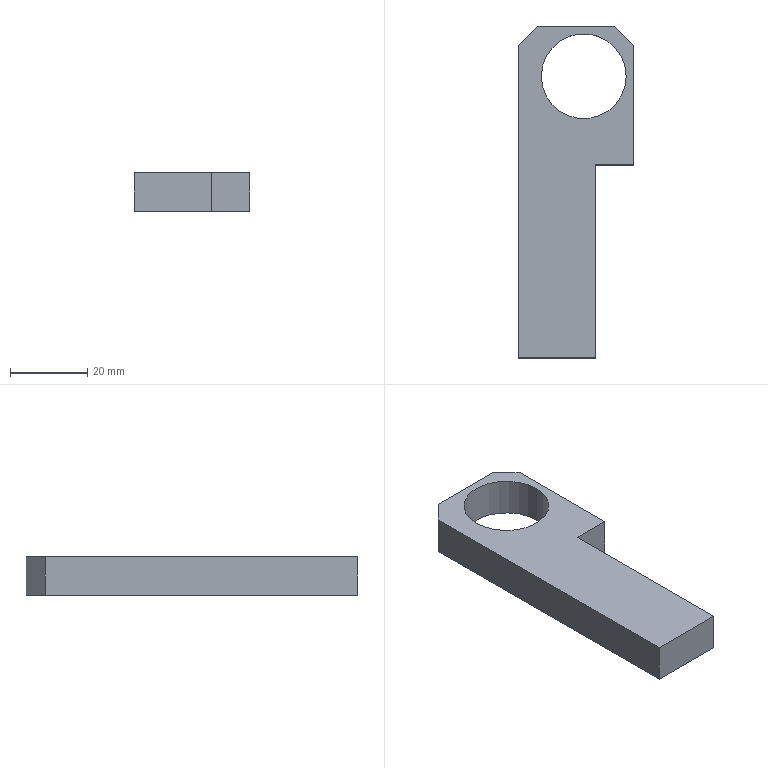Part | STEP file | A08 | 1 solid | 20 faces | box 30 x 86 x 10 mm | volume 16393 mm3 | plane 10 | cylinder 6 | cone 4 | commonest cylinder face diameters 4.2 x4 22 x2
STEP:
#1=CARTESIAN_POINT('',(0.,0.,0.));
#2=DIRECTION('',(0.,0.,1.));
#3=DIRECTION('',(1.,0.,0.));
#4=AXIS2_PLACEMENT_3D('',#1,#2,#3);
#5=CARTESIAN_POINT('',(-7.4,-13.,2.9));
#6=VERTEX_POINT('',#5);
#7=CARTESIAN_POINT('',(5.,-13.,2.9));
#8=VERTEX_POINT('',#7);
#9=CARTESIAN_POINT('',(5.,-13.,2.9));
#10=DIRECTION('',(1.,0.,0.));
#11=VECTOR('',#10,1.);
#12=LINE('',#9,#11);
#13=CARTESIAN_POINT('',(5.,-13.,5.));
#14=DIRECTION('',(1.,0.,0.));
#15=DIRECTION('',(0.,0.,-1.));
#16=AXIS2_PLACEMENT_3D('',#13,#14,#15);
#17=CYLINDRICAL_SURFACE('',#16,2.1);
#18=CARTESIAN_POINT('',(6.283,0.));
#19=DIRECTION('',(0.,1.));
#20=VECTOR('',#19,1.);
#21=LINE('',#18,#20);
#22=(GEOMETRIC_REPRESENTATION_CONTEXT(2)PARAMETRIC_REPRESENTATION_CONTEXT()REPRESENTATION_CONTEXT('',''));
#23=DEFINITIONAL_REPRESENTATION('',(#21),#22);
#24=PCURVE('',#17,#23);
#25=CARTESIAN_POINT('',(5.,-13.,5.));
#26=DIRECTION('',(1.,0.,0.));
#27=DIRECTION('',(0.,0.,-1.));
#28=AXIS2_PLACEMENT_3D('',#25,#26,#27);
#29=CYLINDRICAL_SURFACE('',#28,2.1);
#30=CARTESIAN_POINT('',(0.,0.));
#31=DIRECTION('',(0.,1.));
#32=VECTOR('',#31,1.);
#33=LINE('',#30,#32);
#34=(GEOMETRIC_REPRESENTATION_CONTEXT(2)PARAMETRIC_REPRESENTATION_CONTEXT()REPRESENTATION_CONTEXT('',''));
#35=DEFINITIONAL_REPRESENTATION('',(#33),#34);
#36=PCURVE('',#29,#35);
#37=SURFACE_CURVE('',#12,(#24,#36),.PCURVE_S1.);
#38=EDGE_CURVE('',#6,#8,#37,.T.);
#39=ORIENTED_EDGE('',*,*,#38,.T.);
#40=CARTESIAN_POINT('',(5.,-13.,7.1));
#41=VERTEX_POINT('',#40);
#42=CARTESIAN_POINT('',(5.,-13.,5.));
#43=DIRECTION('',(1.,0.,0.));
#44=DIRECTION('',(0.,0.,-1.));
#45=AXIS2_PLACEMENT_3D('',#42,#43,#44);
#46=CIRCLE('',#45,2.1);
#47=CARTESIAN_POINT('',(0.,0.));
#48=DIRECTION('',(1.,0.));
#49=VECTOR('',#48,1.);
#50=LINE('',#47,#49);
#51=(GEOMETRIC_REPRESENTATION_CONTEXT(2)PARAMETRIC_REPRESENTATION_CONTEXT()REPRESENTATION_CONTEXT('',''));
#52=DEFINITIONAL_REPRESENTATION('',(#50),#51);
#53=PCURVE('',#17,#52);
#54=CARTESIAN_POINT('',(5.,-43.,0.));
#55=DIRECTION('',(-1.,0.,0.));
#56=DIRECTION('',(0.,0.,1.));
#57=AXIS2_PLACEMENT_3D('',#54,#55,#56);
#58=PLANE('',#57);
#59=CARTESIAN_POINT('',(2.9,30.));
#60=CARTESIAN_POINT('',(2.9,33.637));
#61=CARTESIAN_POINT('',(6.05,31.819));
#62=CARTESIAN_POINT('',(9.2,30.));
#63=CARTESIAN_POINT('',(6.05,28.181));
#64=CARTESIAN_POINT('',(2.9,26.363));
#65=CARTESIAN_POINT('',(2.9,30.));
#66=(BOUNDED_CURVE()B_SPLINE_CURVE(2,(#59,#60,#61,#62,#63,#64,#65),.UNSPECIFIED.,.T.,.F.)B_SPLINE_CURVE_WITH_KNOTS((1,2,2,2,2,1),(-2.094,0.,2.094,4.189,6.283,8.378),.UNSPECIFIED.)CURVE()GEOMETRIC_REPRESENTATION_ITEM()RATIONAL_B_SPLINE_CURVE((1.,0.5,1.,0.5,1.,0.5,1.))REPRESENTATION_ITEM(''));
#67=(GEOMETRIC_REPRESENTATION_CONTEXT(2)PARAMETRIC_REPRESENTATION_CONTEXT()REPRESENTATION_CONTEXT('',''));
#68=DEFINITIONAL_REPRESENTATION('',(#66),#67);
#69=PCURVE('',#58,#68);
#70=SURFACE_CURVE('',#46,(#53,#69),.PCURVE_S1.);
#71=EDGE_CURVE('',#41,#8,#70,.T.);
#72=ORIENTED_EDGE('',*,*,#71,.F.);
#73=CARTESIAN_POINT('',(-7.4,-13.,7.1));
#74=VERTEX_POINT('',#73);
#75=CARTESIAN_POINT('',(5.,-13.,7.1));
#76=DIRECTION('',(1.,0.,0.));
#77=VECTOR('',#76,1.);
#78=LINE('',#75,#77);
#79=CARTESIAN_POINT('',(3.142,0.));
#80=DIRECTION('',(0.,1.));
#81=VECTOR('',#80,1.);
#82=LINE('',#79,#81);
#83=(GEOMETRIC_REPRESENTATION_CONTEXT(2)PARAMETRIC_REPRESENTATION_CONTEXT()REPRESENTATION_CONTEXT('',''));
#84=DEFINITIONAL_REPRESENTATION('',(#82),#83);
#85=PCURVE('',#17,#84);
#86=CARTESIAN_POINT('',(3.142,0.));
#87=DIRECTION('',(0.,1.));
#88=VECTOR('',#87,1.);
#89=LINE('',#86,#88);
#90=(GEOMETRIC_REPRESENTATION_CONTEXT(2)PARAMETRIC_REPRESENTATION_CONTEXT()REPRESENTATION_CONTEXT('',''));
#91=DEFINITIONAL_REPRESENTATION('',(#89),#90);
#92=PCURVE('',#29,#91);
#93=SURFACE_CURVE('',#78,(#85,#92),.PCURVE_S1.);
#94=EDGE_CURVE('',#74,#41,#93,.T.);
#95=ORIENTED_EDGE('',*,*,#94,.F.);
#96=CARTESIAN_POINT('',(-7.4,-13.,5.));
#97=DIRECTION('',(1.,0.,0.));
#98=DIRECTION('',(0.,0.,-1.));
#99=AXIS2_PLACEMENT_3D('',#96,#97,#98);
#100=CIRCLE('',#99,2.1);
#101=CARTESIAN_POINT('',(0.,-12.4));
#102=DIRECTION('',(1.,0.));
#103=VECTOR('',#102,1.);
#104=LINE('',#101,#103);
#105=(GEOMETRIC_REPRESENTATION_CONTEXT(2)PARAMETRIC_REPRESENTATION_CONTEXT()REPRESENTATION_CONTEXT('',''));
#106=DEFINITIONAL_REPRESENTATION('',(#104),#105);
#107=PCURVE('',#17,#106);
#108=CARTESIAN_POINT('',(-7.4,-13.,5.));
#109=DIRECTION('',(1.,0.,0.));
#110=DIRECTION('',(0.,0.,-1.));
#111=AXIS2_PLACEMENT_3D('',#108,#109,#110);
#112=CONICAL_SURFACE('',#111,2.1,1.03);
#113=CARTESIAN_POINT('',(0.,0.));
#114=DIRECTION('',(1.,0.));
#115=VECTOR('',#114,1.);
#116=LINE('',#113,#115);
#117=(GEOMETRIC_REPRESENTATION_CONTEXT(2)PARAMETRIC_REPRESENTATION_CONTEXT()REPRESENTATION_CONTEXT('',''));
#118=DEFINITIONAL_REPRESENTATION('',(#116),#117);
#119=PCURVE('',#112,#118);
#120=SURFACE_CURVE('',#100,(#107,#119),.PCURVE_S1.);
#121=EDGE_CURVE('',#74,#6,#120,.T.);
#122=ORIENTED_EDGE('',*,*,#121,.T.);
#123=EDGE_LOOP('',(#39,#72,#95,#122));
#124=FACE_BOUND('',#123,.F.);
#125=ADVANCED_FACE('',(#124),#17,.F.);
#126=ORIENTED_EDGE('',*,*,#121,.F.);
#127=CARTESIAN_POINT('',(-8.662,-13.,5.));
#128=VERTEX_POINT('',#127);
#129=CARTESIAN_POINT('',(-7.4,-13.,7.1));
#130=DIRECTION('',(0.515,0.,0.8572));
#131=VECTOR('',#130,1.);
#132=LINE('',#129,#131);
#133=CARTESIAN_POINT('',(3.142,0.));
#134=DIRECTION('',(0.,1.));
#135=VECTOR('',#134,1.);
#136=LINE('',#133,#135);
#137=(GEOMETRIC_REPRESENTATION_CONTEXT(2)PARAMETRIC_REPRESENTATION_CONTEXT()REPRESENTATION_CONTEXT('',''));
#138=DEFINITIONAL_REPRESENTATION('',(#136),#137);
#139=PCURVE('',#112,#138);
#140=CARTESIAN_POINT('',(-7.4,-13.,5.));
#141=DIRECTION('',(1.,0.,0.));
#142=DIRECTION('',(0.,0.,-1.));
#143=AXIS2_PLACEMENT_3D('',#140,#141,#142);
#144=CONICAL_SURFACE('',#143,2.1,1.03);
#145=CARTESIAN_POINT('',(3.142,0.));
#146=DIRECTION('',(0.,1.));
#147=VECTOR('',#146,1.);
#148=LINE('',#145,#147);
#149=(GEOMETRIC_REPRESENTATION_CONTEXT(2)PARAMETRIC_REPRESENTATION_CONTEXT()REPRESENTATION_CONTEXT('',''));
#150=DEFINITIONAL_REPRESENTATION('',(#148),#149);
#151=PCURVE('',#144,#150);
#152=SURFACE_CURVE('',#132,(#139,#151),.PCURVE_S1.);
#153=EDGE_CURVE('',#128,#74,#152,.T.);
#154=ORIENTED_EDGE('',*,*,#153,.F.);
#155=CARTESIAN_POINT('',(-7.4,-13.,2.9));
#156=DIRECTION('',(0.515,0.,-0.8572));
#157=VECTOR('',#156,1.);
#158=LINE('',#155,#157);
#159=CARTESIAN_POINT('',(6.283,0.));
#160=DIRECTION('',(0.,1.));
#161=VECTOR('',#160,1.);
#162=LINE('',#159,#161);
#163=(GEOMETRIC_REPRESENTATION_CONTEXT(2)PARAMETRIC_REPRESENTATION_CONTEXT()REPRESENTATION_CONTEXT('',''));
#164=DEFINITIONAL_REPRESENTATION('',(#162),#163);
#165=PCURVE('',#112,#164);
#166=CARTESIAN_POINT('',(0.,0.));
#167=DIRECTION('',(0.,1.));
#168=VECTOR('',#167,1.);
#169=LINE('',#166,#168);
#170=(GEOMETRIC_REPRESENTATION_CONTEXT(2)PARAMETRIC_REPRESENTATION_CONTEXT()REPRESENTATION_CONTEXT('',''));
#171=DEFINITIONAL_REPRESENTATION('',(#169),#170);
#172=PCURVE('',#144,#171);
#173=SURFACE_CURVE('',#158,(#165,#172),.PCURVE_S1.);
#174=EDGE_CURVE('',#128,#6,#173,.T.);
#175=ORIENTED_EDGE('',*,*,#174,.T.);
#176=EDGE_LOOP('',(#126,#154,#175));
#177=FACE_BOUND('',#176,.F.);
#178=ADVANCED_FACE('',(#177),#112,.F.);
#179=CARTESIAN_POINT('',(-7.4,-38.,2.9));
#180=VERTEX_POINT('',#179);
#181=CARTESIAN_POINT('',(5.,-38.,2.9));
#182=VERTEX_POINT('',#181);
#183=CARTESIAN_POINT('',(5.,-38.,2.9));
#184=DIRECTION('',(1.,0.,0.));
#185=VECTOR('',#184,1.);
#186=LINE('',#183,#185);
#187=CARTESIAN_POINT('',(5.,-38.,5.));
#188=DIRECTION('',(1.,0.,0.));
#189=DIRECTION('',(0.,0.,-1.));
#190=AXIS2_PLACEMENT_3D('',#187,#188,#189);
#191=CYLINDRICAL_SURFACE('',#190,2.1);
#192=CARTESIAN_POINT('',(6.283,0.));
#193=DIRECTION('',(0.,1.));
#194=VECTOR('',#193,1.);
#195=LINE('',#192,#194);
#196=(GEOMETRIC_REPRESENTATION_CONTEXT(2)PARAMETRIC_REPRESENTATION_CONTEXT()REPRESENTATION_CONTEXT('',''));
#197=DEFINITIONAL_REPRESENTATION('',(#195),#196);
#198=PCURVE('',#191,#197);
#199=CARTESIAN_POINT('',(5.,-38.,5.));
#200=DIRECTION('',(1.,0.,0.));
#201=DIRECTION('',(0.,0.,-1.));
#202=AXIS2_PLACEMENT_3D('',#199,#200,#201);
#203=CYLINDRICAL_SURFACE('',#202,2.1);
#204=CARTESIAN_POINT('',(0.,0.));
#205=DIRECTION('',(0.,1.));
#206=VECTOR('',#205,1.);
#207=LINE('',#204,#206);
#208=(GEOMETRIC_REPRESENTATION_CONTEXT(2)PARAMETRIC_REPRESENTATION_CONTEXT()REPRESENTATION_CONTEXT('',''));
#209=DEFINITIONAL_REPRESENTATION('',(#207),#208);
#210=PCURVE('',#203,#209);
#211=SURFACE_CURVE('',#186,(#198,#210),.PCURVE_S1.);
#212=EDGE_CURVE('',#180,#182,#211,.T.);
#213=ORIENTED_EDGE('',*,*,#212,.T.);
#214=CARTESIAN_POINT('',(5.,-38.,7.1));
#215=VERTEX_POINT('',#214);
#216=CARTESIAN_POINT('',(5.,-38.,5.));
#217=DIRECTION('',(1.,0.,0.));
#218=DIRECTION('',(0.,0.,-1.));
#219=AXIS2_PLACEMENT_3D('',#216,#217,#218);
#220=CIRCLE('',#219,2.1);
#221=CARTESIAN_POINT('',(0.,0.));
#222=DIRECTION('',(1.,0.));
#223=VECTOR('',#222,1.);
#224=LINE('',#221,#223);
#225=(GEOMETRIC_REPRESENTATION_CONTEXT(2)PARAMETRIC_REPRESENTATION_CONTEXT()REPRESENTATION_CONTEXT('',''));
#226=DEFINITIONAL_REPRESENTATION('',(#224),#225);
#227=PCURVE('',#191,#226);
#228=CARTESIAN_POINT('',(2.9,5.));
#229=CARTESIAN_POINT('',(2.9,8.637));
#230=CARTESIAN_POINT('',(6.05,6.819));
#231=CARTESIAN_POINT('',(9.2,5.));
#232=CARTESIAN_POINT('',(6.05,3.181));
#233=CARTESIAN_POINT('',(2.9,1.363));
#234=CARTESIAN_POINT('',(2.9,5.));
#235=(BOUNDED_CURVE()B_SPLINE_CURVE(2,(#228,#229,#230,#231,#232,#233,#234),.UNSPECIFIED.,.T.,.F.)B_SPLINE_CURVE_WITH_KNOTS((1,2,2,2,2,1),(-2.094,0.,2.094,4.189,6.283,8.378),.UNSPECIFIED.)CURVE()GEOMETRIC_REPRESENTATION_ITEM()RATIONAL_B_SPLINE_CURVE((1.,0.5,1.,0.5,1.,0.5,1.))REPRESENTATION_ITEM(''));
#236=(GEOMETRIC_REPRESENTATION_CONTEXT(2)PARAMETRIC_REPRESENTATION_CONTEXT()REPRESENTATION_CONTEXT('',''));
#237=DEFINITIONAL_REPRESENTATION('',(#235),#236);
#238=PCURVE('',#58,#237);
#239=SURFACE_CURVE('',#220,(#227,#238),.PCURVE_S1.);
#240=EDGE_CURVE('',#215,#182,#239,.T.);
#241=ORIENTED_EDGE('',*,*,#240,.F.);
#242=CARTESIAN_POINT('',(-7.4,-38.,7.1));
#243=VERTEX_POINT('',#242);
#244=CARTESIAN_POINT('',(5.,-38.,7.1));
#245=DIRECTION('',(1.,0.,0.));
#246=VECTOR('',#245,1.);
#247=LINE('',#244,#246);
#248=CARTESIAN_POINT('',(3.142,0.));
#249=DIRECTION('',(0.,1.));
#250=VECTOR('',#249,1.);
#251=LINE('',#248,#250);
#252=(GEOMETRIC_REPRESENTATION_CONTEXT(2)PARAMETRIC_REPRESENTATION_CONTEXT()REPRESENTATION_CONTEXT('',''));
#253=DEFINITIONAL_REPRESENTATION('',(#251),#252);
#254=PCURVE('',#191,#253);
#255=CARTESIAN_POINT('',(3.142,0.));
#256=DIRECTION('',(0.,1.));
#257=VECTOR('',#256,1.);
#258=LINE('',#255,#257);
#259=(GEOMETRIC_REPRESENTATION_CONTEXT(2)PARAMETRIC_REPRESENTATION_CONTEXT()REPRESENTATION_CONTEXT('',''));
#260=DEFINITIONAL_REPRESENTATION('',(#258),#259);
#261=PCURVE('',#203,#260);
#262=SURFACE_CURVE('',#247,(#254,#261),.PCURVE_S1.);
#263=EDGE_CURVE('',#243,#215,#262,.T.);
#264=ORIENTED_EDGE('',*,*,#263,.F.);
#265=CARTESIAN_POINT('',(-7.4,-38.,5.));
#266=DIRECTION('',(1.,0.,0.));
#267=DIRECTION('',(0.,0.,-1.));
#268=AXIS2_PLACEMENT_3D('',#265,#266,#267);
#269=CIRCLE('',#268,2.1);
#270=CARTESIAN_POINT('',(0.,-12.4));
#271=DIRECTION('',(1.,0.));
#272=VECTOR('',#271,1.);
#273=LINE('',#270,#272);
#274=(GEOMETRIC_REPRESENTATION_CONTEXT(2)PARAMETRIC_REPRESENTATION_CONTEXT()REPRESENTATION_CONTEXT('',''));
#275=DEFINITIONAL_REPRESENTATION('',(#273),#274);
#276=PCURVE('',#191,#275);
#277=CARTESIAN_POINT('',(-7.4,-38.,5.));
#278=DIRECTION('',(1.,0.,0.));
#279=DIRECTION('',(0.,0.,-1.));
#280=AXIS2_PLACEMENT_3D('',#277,#278,#279);
#281=CONICAL_SURFACE('',#280,2.1,1.03);
#282=CARTESIAN_POINT('',(0.,0.));
#283=DIRECTION('',(1.,0.));
#284=VECTOR('',#283,1.);
#285=LINE('',#282,#284);
#286=(GEOMETRIC_REPRESENTATION_CONTEXT(2)PARAMETRIC_REPRESENTATION_CONTEXT()REPRESENTATION_CONTEXT('',''));
#287=DEFINITIONAL_REPRESENTATION('',(#285),#286);
#288=PCURVE('',#281,#287);
#289=SURFACE_CURVE('',#269,(#276,#288),.PCURVE_S1.);
#290=EDGE_CURVE('',#243,#180,#289,.T.);
#291=ORIENTED_EDGE('',*,*,#290,.T.);
#292=EDGE_LOOP('',(#213,#241,#264,#291));
#293=FACE_BOUND('',#292,.F.);
#294=ADVANCED_FACE('',(#293),#191,.F.);
#295=ORIENTED_EDGE('',*,*,#290,.F.);
#296=CARTESIAN_POINT('',(-8.662,-38.,5.));
#297=VERTEX_POINT('',#296);
#298=CARTESIAN_POINT('',(-7.4,-38.,7.1));
#299=DIRECTION('',(0.515,0.,0.8572));
#300=VECTOR('',#299,1.);
#301=LINE('',#298,#300);
#302=CARTESIAN_POINT('',(3.142,-1.262));
#303=CARTESIAN_POINT('',(3.142,-1.243));
#304=CARTESIAN_POINT('',(3.142,-1.204));
#305=CARTESIAN_POINT('',(3.142,-1.147));
#306=CARTESIAN_POINT('',(3.142,-1.09));
#307=CARTESIAN_POINT('',(3.142,-1.032));
#308=CARTESIAN_POINT('',(3.142,-0.975));
#309=CARTESIAN_POINT('',(3.142,-0.9177));
#310=CARTESIAN_POINT('',(3.142,-0.8603));
#311=CARTESIAN_POINT('',(3.142,-0.803));
#312=CARTESIAN_POINT('',(3.142,-0.7456));
#313=CARTESIAN_POINT('',(3.142,-0.6883));
#314=CARTESIAN_POINT('',(3.142,-0.6309));
#315=CARTESIAN_POINT('',(3.142,-0.5735));
#316=CARTESIAN_POINT('',(3.142,-0.5162));
#317=CARTESIAN_POINT('',(3.142,-0.4588));
#318=CARTESIAN_POINT('',(3.142,-0.4015));
#319=CARTESIAN_POINT('',(3.142,-0.3441));
#320=CARTESIAN_POINT('',(3.142,-0.2868));
#321=CARTESIAN_POINT('',(3.142,-0.2294));
#322=CARTESIAN_POINT('',(3.142,-0.1721));
#323=CARTESIAN_POINT('',(3.142,-0.1147));
#324=CARTESIAN_POINT('',(3.142,-0.05735));
#325=CARTESIAN_POINT('',(3.142,-0.01912));
#326=CARTESIAN_POINT('',(3.142,0.));
#327=B_SPLINE_CURVE_WITH_KNOTS('',3,(#302,#303,#304,#305,#306,#307,#308,#309,#310,#311,#312,#313,#314,#315,#316,#317,#318,#319,#320,#321,#322,#323,#324,#325,#326),.UNSPECIFIED.,.F.,.F.,(4,1,1,1,1,1,1,1,1,1,1,1,1,1,1,1,1,1,1,1,1,1,4),(-2.45,-2.339,-2.227,-2.116,-2.004,-1.893,-1.782,-1.67,-1.559,-1.448,-1.336,-1.225,-1.114,-1.002,-0.8909,-0.7795,-0.6682,-0.5568,-0.4454,-0.3341,-0.2227,-0.1114,0.),.UNSPECIFIED.);
#328=(GEOMETRIC_REPRESENTATION_CONTEXT(2)PARAMETRIC_REPRESENTATION_CONTEXT()REPRESENTATION_CONTEXT('',''));
#329=DEFINITIONAL_REPRESENTATION('',(#327),#328);
#330=PCURVE('',#281,#329);
#331=CARTESIAN_POINT('',(-7.4,-38.,5.));
#332=DIRECTION('',(1.,0.,0.));
#333=DIRECTION('',(0.,0.,-1.));
#334=AXIS2_PLACEMENT_3D('',#331,#332,#333);
#335=CONICAL_SURFACE('',#334,2.1,1.03);
#336=CARTESIAN_POINT('',(3.142,-1.262));
#337=CARTESIAN_POINT('',(3.142,-1.243));
#338=CARTESIAN_POINT('',(3.142,-1.204));
#339=CARTESIAN_POINT('',(3.142,-1.147));
#340=CARTESIAN_POINT('',(3.142,-1.09));
#341=CARTESIAN_POINT('',(3.142,-1.032));
#342=CARTESIAN_POINT('',(3.142,-0.975));
#343=CARTESIAN_POINT('',(3.142,-0.9177));
#344=CARTESIAN_POINT('',(3.142,-0.8603));
#345=CARTESIAN_POINT('',(3.142,-0.803));
#346=CARTESIAN_POINT('',(3.142,-0.7456));
#347=CARTESIAN_POINT('',(3.142,-0.6883));
#348=CARTESIAN_POINT('',(3.142,-0.6309));
#349=CARTESIAN_POINT('',(3.142,-0.5735));
#350=CARTESIAN_POINT('',(3.142,-0.5162));
#351=CARTESIAN_POINT('',(3.142,-0.4588));
#352=CARTESIAN_POINT('',(3.142,-0.4015));
#353=CARTESIAN_POINT('',(3.142,-0.3441));
#354=CARTESIAN_POINT('',(3.142,-0.2868));
#355=CARTESIAN_POINT('',(3.142,-0.2294));
#356=CARTESIAN_POINT('',(3.142,-0.1721));
#357=CARTESIAN_POINT('',(3.142,-0.1147));
#358=CARTESIAN_POINT('',(3.142,-0.05735));
#359=CARTESIAN_POINT('',(3.142,-0.01912));
#360=CARTESIAN_POINT('',(3.142,0.));
#361=B_SPLINE_CURVE_WITH_KNOTS('',3,(#336,#337,#338,#339,#340,#341,#342,#343,#344,#345,#346,#347,#348,#349,#350,#351,#352,#353,#354,#355,#356,#357,#358,#359,#360),.UNSPECIFIED.,.F.,.F.,(4,1,1,1,1,1,1,1,1,1,1,1,1,1,1,1,1,1,1,1,1,1,4),(-2.45,-2.339,-2.227,-2.116,-2.004,-1.893,-1.782,-1.67,-1.559,-1.448,-1.336,-1.225,-1.114,-1.002,-0.8909,-0.7795,-0.6682,-0.5568,-0.4454,-0.3341,-0.2227,-0.1114,0.),.UNSPECIFIED.);
#362=(GEOMETRIC_REPRESENTATION_CONTEXT(2)PARAMETRIC_REPRESENTATION_CONTEXT()REPRESENTATION_CONTEXT('',''));
#363=DEFINITIONAL_REPRESENTATION('',(#361),#362);
#364=PCURVE('',#335,#363);
#365=SURFACE_CURVE('',#301,(#330,#364),.PCURVE_S1.);
#366=EDGE_CURVE('',#297,#243,#365,.T.);
#367=ORIENTED_EDGE('',*,*,#366,.F.);
#368=CARTESIAN_POINT('',(-7.4,-38.,2.9));
#369=DIRECTION('',(0.515,0.,-0.8572));
#370=VECTOR('',#369,1.);
#371=LINE('',#368,#370);
#372=CARTESIAN_POINT('',(6.283,0.));
#373=DIRECTION('',(0.,1.));
#374=VECTOR('',#373,1.);
#375=LINE('',#372,#374);
#376=(GEOMETRIC_REPRESENTATION_CONTEXT(2)PARAMETRIC_REPRESENTATION_CONTEXT()REPRESENTATION_CONTEXT('',''));
#377=DEFINITIONAL_REPRESENTATION('',(#375),#376);
#378=PCURVE('',#281,#377);
#379=CARTESIAN_POINT('',(0.,0.));
#380=DIRECTION('',(0.,1.));
#381=VECTOR('',#380,1.);
#382=LINE('',#379,#381);
#383=(GEOMETRIC_REPRESENTATION_CONTEXT(2)PARAMETRIC_REPRESENTATION_CONTEXT()REPRESENTATION_CONTEXT('',''));
#384=DEFINITIONAL_REPRESENTATION('',(#382),#383);
#385=PCURVE('',#335,#384);
#386=SURFACE_CURVE('',#371,(#378,#385),.PCURVE_S1.);
#387=EDGE_CURVE('',#297,#180,#386,.T.);
#388=ORIENTED_EDGE('',*,*,#387,.T.);
#389=EDGE_LOOP('',(#295,#367,#388));
#390=FACE_BOUND('',#389,.F.);
#391=ADVANCED_FACE('',(#390),#281,.F.);
#392=CARTESIAN_POINT('',(13.,30.,0.));
#393=VERTEX_POINT('',#392);
#394=CARTESIAN_POINT('',(13.,30.,10.));
#395=VERTEX_POINT('',#394);
#396=CARTESIAN_POINT('',(13.,30.,0.));
#397=DIRECTION('',(0.,0.,1.));
#398=VECTOR('',#397,1.);
#399=LINE('',#396,#398);
#400=CARTESIAN_POINT('',(2.,30.,0.));
#401=DIRECTION('',(0.,0.,1.));
#402=DIRECTION('',(1.,0.,0.));
#403=AXIS2_PLACEMENT_3D('',#400,#401,#402);
#404=CYLINDRICAL_SURFACE('',#403,11.);
#405=CARTESIAN_POINT('',(6.283,0.));
#406=DIRECTION('',(0.,1.));
#407=VECTOR('',#406,1.);
#408=LINE('',#405,#407);
#409=(GEOMETRIC_REPRESENTATION_CONTEXT(2)PARAMETRIC_REPRESENTATION_CONTEXT()REPRESENTATION_CONTEXT('',''));
#410=DEFINITIONAL_REPRESENTATION('',(#408),#409);
#411=PCURVE('',#404,#410);
#412=CARTESIAN_POINT('',(2.,30.,0.));
#413=DIRECTION('',(0.,0.,1.));
#414=DIRECTION('',(1.,0.,0.));
#415=AXIS2_PLACEMENT_3D('',#412,#413,#414);
#416=CYLINDRICAL_SURFACE('',#415,11.);
#417=CARTESIAN_POINT('',(0.,0.));
#418=DIRECTION('',(0.,1.));
#419=VECTOR('',#418,1.);
#420=LINE('',#417,#419);
#421=(GEOMETRIC_REPRESENTATION_CONTEXT(2)PARAMETRIC_REPRESENTATION_CONTEXT()REPRESENTATION_CONTEXT('',''));
#422=DEFINITIONAL_REPRESENTATION('',(#420),#421);
#423=PCURVE('',#416,#422);
#424=SURFACE_CURVE('',#399,(#411,#423),.PCURVE_S1.);
#425=EDGE_CURVE('',#393,#395,#424,.T.);
#426=ORIENTED_EDGE('',*,*,#425,.T.);
#427=CARTESIAN_POINT('',(-9.,30.,10.));
#428=VERTEX_POINT('',#427);
#429=CARTESIAN_POINT('',(2.,30.,10.));
#430=DIRECTION('',(0.,0.,1.));
#431=DIRECTION('',(1.,0.,0.));
#432=AXIS2_PLACEMENT_3D('',#429,#430,#431);
#433=CIRCLE('',#432,11.);
#434=CARTESIAN_POINT('',(0.,10.));
#435=DIRECTION('',(1.,0.));
#436=VECTOR('',#435,1.);
#437=LINE('',#434,#436);
#438=(GEOMETRIC_REPRESENTATION_CONTEXT(2)PARAMETRIC_REPRESENTATION_CONTEXT()REPRESENTATION_CONTEXT('',''));
#439=DEFINITIONAL_REPRESENTATION('',(#437),#438);
#440=PCURVE('',#404,#439);
#441=CARTESIAN_POINT('',(0.,0.,10.));
#442=DIRECTION('',(0.,0.,1.));
#443=DIRECTION('',(1.,0.,0.));
#444=AXIS2_PLACEMENT_3D('',#441,#442,#443);
#445=PLANE('',#444);
#446=CARTESIAN_POINT('',(2.,30.));
#447=DIRECTION('',(1.,0.));
#448=AXIS2_PLACEMENT_2D('',#446,#447);
#449=CIRCLE('',#448,11.);
#450=(GEOMETRIC_REPRESENTATION_CONTEXT(2)PARAMETRIC_REPRESENTATION_CONTEXT()REPRESENTATION_CONTEXT('',''));
#451=DEFINITIONAL_REPRESENTATION('',(#449),#450);
#452=PCURVE('',#445,#451);
#453=SURFACE_CURVE('',#433,(#440,#452),.PCURVE_S1.);
#454=EDGE_CURVE('',#428,#395,#453,.T.);
#455=ORIENTED_EDGE('',*,*,#454,.F.);
#456=CARTESIAN_POINT('',(-9.,30.,0.));
#457=VERTEX_POINT('',#456);
#458=CARTESIAN_POINT('',(-9.,30.,0.));
#459=DIRECTION('',(0.,0.,1.));
#460=VECTOR('',#459,1.);
#461=LINE('',#458,#460);
#462=CARTESIAN_POINT('',(3.142,0.));
#463=DIRECTION('',(0.,1.));
#464=VECTOR('',#463,1.);
#465=LINE('',#462,#464);
#466=(GEOMETRIC_REPRESENTATION_CONTEXT(2)PARAMETRIC_REPRESENTATION_CONTEXT()REPRESENTATION_CONTEXT('',''));
#467=DEFINITIONAL_REPRESENTATION('',(#465),#466);
#468=PCURVE('',#404,#467);
#469=CARTESIAN_POINT('',(3.142,0.));
#470=DIRECTION('',(0.,1.));
#471=VECTOR('',#470,1.);
#472=LINE('',#469,#471);
#473=(GEOMETRIC_REPRESENTATION_CONTEXT(2)PARAMETRIC_REPRESENTATION_CONTEXT()REPRESENTATION_CONTEXT('',''));
#474=DEFINITIONAL_REPRESENTATION('',(#472),#473);
#475=PCURVE('',#416,#474);
#476=SURFACE_CURVE('',#461,(#468,#475),.PCURVE_S1.);
#477=EDGE_CURVE('',#457,#428,#476,.T.);
#478=ORIENTED_EDGE('',*,*,#477,.F.);
#479=CARTESIAN_POINT('',(2.,30.,0.));
#480=DIRECTION('',(0.,0.,1.));
#481=DIRECTION('',(1.,0.,0.));
#482=AXIS2_PLACEMENT_3D('',#479,#480,#481);
#483=CIRCLE('',#482,11.);
#484=CARTESIAN_POINT('',(0.,0.));
#485=DIRECTION('',(1.,0.));
#486=VECTOR('',#485,1.);
#487=LINE('',#484,#486);
#488=(GEOMETRIC_REPRESENTATION_CONTEXT(2)PARAMETRIC_REPRESENTATION_CONTEXT()REPRESENTATION_CONTEXT('',''));
#489=DEFINITIONAL_REPRESENTATION('',(#487),#488);
#490=PCURVE('',#404,#489);
#491=CARTESIAN_POINT('',(0.,0.,0.));
#492=DIRECTION('',(0.,0.,1.));
#493=DIRECTION('',(1.,0.,0.));
#494=AXIS2_PLACEMENT_3D('',#491,#492,#493);
#495=PLANE('',#494);
#496=CARTESIAN_POINT('',(2.,30.));
#497=DIRECTION('',(1.,0.));
#498=AXIS2_PLACEMENT_2D('',#496,#497);
#499=CIRCLE('',#498,11.);
#500=(GEOMETRIC_REPRESENTATION_CONTEXT(2)PARAMETRIC_REPRESENTATION_CONTEXT()REPRESENTATION_CONTEXT('',''));
#501=DEFINITIONAL_REPRESENTATION('',(#499),#500);
#502=PCURVE('',#495,#501);
#503=SURFACE_CURVE('',#483,(#490,#502),.PCURVE_S1.);
#504=EDGE_CURVE('',#457,#393,#503,.T.);
#505=ORIENTED_EDGE('',*,*,#504,.T.);
#506=EDGE_LOOP('',(#426,#455,#478,#505));
#507=FACE_BOUND('',#506,.F.);
#508=ADVANCED_FACE('',(#507),#404,.F.);
#509=CARTESIAN_POINT('',(15.,7.,0.));
#510=VERTEX_POINT('',#509);
#511=CARTESIAN_POINT('',(15.,38.,0.));
#512=VERTEX_POINT('',#511);
#513=CARTESIAN_POINT('',(15.,43.,0.));
#514=DIRECTION('',(0.,1.,0.));
#515=VECTOR('',#514,1.);
#516=LINE('',#513,#515);
#517=CARTESIAN_POINT('',(15.,43.,10.));
#518=DIRECTION('',(-1.,0.,0.));
#519=DIRECTION('',(0.,-1.,0.));
#520=AXIS2_PLACEMENT_3D('',#517,#518,#519);
#521=PLANE('',#520);
#522=CARTESIAN_POINT('',(0.,-10.));
#523=DIRECTION('',(-1.,0.));
#524=VECTOR('',#523,1.);
#525=LINE('',#522,#524);
#526=(GEOMETRIC_REPRESENTATION_CONTEXT(2)PARAMETRIC_REPRESENTATION_CONTEXT()REPRESENTATION_CONTEXT('',''));
#527=DEFINITIONAL_REPRESENTATION('',(#525),#526);
#528=PCURVE('',#521,#527);
#529=CARTESIAN_POINT('',(15.,43.));
#530=DIRECTION('',(0.,1.));
#531=VECTOR('',#530,1.);
#532=LINE('',#529,#531);
#533=(GEOMETRIC_REPRESENTATION_CONTEXT(2)PARAMETRIC_REPRESENTATION_CONTEXT()REPRESENTATION_CONTEXT('',''));
#534=DEFINITIONAL_REPRESENTATION('',(#532),#533);
#535=PCURVE('',#495,#534);
#536=SURFACE_CURVE('',#516,(#528,#535),.PCURVE_S1.);
#537=EDGE_CURVE('',#510,#512,#536,.T.);
#538=ORIENTED_EDGE('',*,*,#537,.T.);
#539=CARTESIAN_POINT('',(15.,38.,10.));
#540=VERTEX_POINT('',#539);
#541=CARTESIAN_POINT('',(15.,38.,10.));
#542=DIRECTION('',(0.,0.,1.));
#543=VECTOR('',#542,1.);
#544=LINE('',#541,#543);
#545=CARTESIAN_POINT('',(5.,0.));
#546=DIRECTION('',(0.,1.));
#547=VECTOR('',#546,1.);
#548=LINE('',#545,#547);
#549=(GEOMETRIC_REPRESENTATION_CONTEXT(2)PARAMETRIC_REPRESENTATION_CONTEXT()REPRESENTATION_CONTEXT('',''));
#550=DEFINITIONAL_REPRESENTATION('',(#548),#549);
#551=PCURVE('',#521,#550);
#552=CARTESIAN_POINT('',(10.,43.,10.));
#553=DIRECTION('',(-0.7071,-0.7071,0.));
#554=DIRECTION('',(0.,0.,-1.));
#555=AXIS2_PLACEMENT_3D('',#552,#553,#554);
#556=PLANE('',#555);
#557=CARTESIAN_POINT('',(0.,7.071));
#558=DIRECTION('',(-1.,0.));
#559=VECTOR('',#558,1.);
#560=LINE('',#557,#559);
#561=(GEOMETRIC_REPRESENTATION_CONTEXT(2)PARAMETRIC_REPRESENTATION_CONTEXT()REPRESENTATION_CONTEXT('',''));
#562=DEFINITIONAL_REPRESENTATION('',(#560),#561);
#563=PCURVE('',#556,#562);
#564=SURFACE_CURVE('',#544,(#551,#563),.PCURVE_S1.);
#565=EDGE_CURVE('',#512,#540,#564,.T.);
#566=ORIENTED_EDGE('',*,*,#565,.T.);
#567=CARTESIAN_POINT('',(15.,7.,10.));
#568=VERTEX_POINT('',#567);
#569=CARTESIAN_POINT('',(15.,43.,10.));
#570=DIRECTION('',(0.,1.,0.));
#571=VECTOR('',#570,1.);
#572=LINE('',#569,#571);
#573=CARTESIAN_POINT('',(0.,0.));
#574=DIRECTION('',(-1.,0.));
#575=VECTOR('',#574,1.);
#576=LINE('',#573,#575);
#577=(GEOMETRIC_REPRESENTATION_CONTEXT(2)PARAMETRIC_REPRESENTATION_CONTEXT()REPRESENTATION_CONTEXT('',''));
#578=DEFINITIONAL_REPRESENTATION('',(#576),#577);
#579=PCURVE('',#521,#578);
#580=CARTESIAN_POINT('',(15.,43.));
#581=DIRECTION('',(0.,1.));
#582=VECTOR('',#581,1.);
#583=LINE('',#580,#582);
#584=(GEOMETRIC_REPRESENTATION_CONTEXT(2)PARAMETRIC_REPRESENTATION_CONTEXT()REPRESENTATION_CONTEXT('',''));
#585=DEFINITIONAL_REPRESENTATION('',(#583),#584);
#586=PCURVE('',#445,#585);
#587=SURFACE_CURVE('',#572,(#579,#586),.PCURVE_S1.);
#588=EDGE_CURVE('',#568,#540,#587,.T.);
#589=ORIENTED_EDGE('',*,*,#588,.F.);
#590=CARTESIAN_POINT('',(15.,7.,0.));
#591=DIRECTION('',(0.,0.,1.));
#592=VECTOR('',#591,1.);
#593=LINE('',#590,#592);
#594=CARTESIAN_POINT('',(36.,-10.));
#595=DIRECTION('',(0.,1.));
#596=VECTOR('',#595,1.);
#597=LINE('',#594,#596);
#598=(GEOMETRIC_REPRESENTATION_CONTEXT(2)PARAMETRIC_REPRESENTATION_CONTEXT()REPRESENTATION_CONTEXT('',''));
#599=DEFINITIONAL_REPRESENTATION('',(#597),#598);
#600=PCURVE('',#521,#599);
#601=CARTESIAN_POINT('',(15.,7.,0.));
#602=DIRECTION('',(0.,1.,0.));
#603=DIRECTION('',(0.,0.,1.));
#604=AXIS2_PLACEMENT_3D('',#601,#602,#603);
#605=PLANE('',#604);
#606=CARTESIAN_POINT('',(0.,0.));
#607=DIRECTION('',(1.,0.));
#608=VECTOR('',#607,1.);
#609=LINE('',#606,#608);
#610=(GEOMETRIC_REPRESENTATION_CONTEXT(2)PARAMETRIC_REPRESENTATION_CONTEXT()REPRESENTATION_CONTEXT('',''));
#611=DEFINITIONAL_REPRESENTATION('',(#609),#610);
#612=PCURVE('',#605,#611);
#613=SURFACE_CURVE('',#593,(#600,#612),.PCURVE_S1.);
#614=EDGE_CURVE('',#510,#568,#613,.T.);
#615=ORIENTED_EDGE('',*,*,#614,.F.);
#616=EDGE_LOOP('',(#538,#566,#589,#615));
#617=FACE_BOUND('',#616,.T.);
#618=ADVANCED_FACE('',(#617),#521,.F.);
#619=CARTESIAN_POINT('',(10.,43.,10.));
#620=VERTEX_POINT('',#619);
#621=CARTESIAN_POINT('',(-10.,43.,10.));
#622=VERTEX_POINT('',#621);
#623=CARTESIAN_POINT('',(-15.,43.,10.));
#624=DIRECTION('',(-1.,0.,0.));
#625=VECTOR('',#624,1.);
#626=LINE('',#623,#625);
#627=CARTESIAN_POINT('',(-15.,43.,10.));
#628=DIRECTION('',(0.,-1.,0.));
#629=DIRECTION('',(0.,0.,-1.));
#630=AXIS2_PLACEMENT_3D('',#627,#628,#629);
#631=PLANE('',#630);
#632=CARTESIAN_POINT('',(0.,0.));
#633=DIRECTION('',(0.,-1.));
#634=VECTOR('',#633,1.);
#635=LINE('',#632,#634);
#636=(GEOMETRIC_REPRESENTATION_CONTEXT(2)PARAMETRIC_REPRESENTATION_CONTEXT()REPRESENTATION_CONTEXT('',''));
#637=DEFINITIONAL_REPRESENTATION('',(#635),#636);
#638=PCURVE('',#631,#637);
#639=CARTESIAN_POINT('',(-15.,43.));
#640=DIRECTION('',(-1.,0.));
#641=VECTOR('',#640,1.);
#642=LINE('',#639,#641);
#643=(GEOMETRIC_REPRESENTATION_CONTEXT(2)PARAMETRIC_REPRESENTATION_CONTEXT()REPRESENTATION_CONTEXT('',''));
#644=DEFINITIONAL_REPRESENTATION('',(#642),#643);
#645=PCURVE('',#445,#644);
#646=SURFACE_CURVE('',#626,(#638,#645),.PCURVE_S1.);
#647=EDGE_CURVE('',#620,#622,#646,.T.);
#648=ORIENTED_EDGE('',*,*,#647,.F.);
#649=CARTESIAN_POINT('',(10.,43.,0.));
#650=VERTEX_POINT('',#649);
#651=CARTESIAN_POINT('',(10.,43.,10.));
#652=DIRECTION('',(0.,0.,-1.));
#653=VECTOR('',#652,1.);
#654=LINE('',#651,#653);
#655=CARTESIAN_POINT('',(0.,25.));
#656=DIRECTION('',(1.,0.));
#657=VECTOR('',#656,1.);
#658=LINE('',#655,#657);
#659=(GEOMETRIC_REPRESENTATION_CONTEXT(2)PARAMETRIC_REPRESENTATION_CONTEXT()REPRESENTATION_CONTEXT('',''));
#660=DEFINITIONAL_REPRESENTATION('',(#658),#659);
#661=PCURVE('',#631,#660);
#662=CARTESIAN_POINT('',(0.,0.));
#663=DIRECTION('',(1.,0.));
#664=VECTOR('',#663,1.);
#665=LINE('',#662,#664);
#666=(GEOMETRIC_REPRESENTATION_CONTEXT(2)PARAMETRIC_REPRESENTATION_CONTEXT()REPRESENTATION_CONTEXT('',''));
#667=DEFINITIONAL_REPRESENTATION('',(#665),#666);
#668=PCURVE('',#556,#667);
#669=SURFACE_CURVE('',#654,(#661,#668),.PCURVE_S1.);
#670=EDGE_CURVE('',#620,#650,#669,.T.);
#671=ORIENTED_EDGE('',*,*,#670,.T.);
#672=CARTESIAN_POINT('',(-10.,43.,0.));
#673=VERTEX_POINT('',#672);
#674=CARTESIAN_POINT('',(-15.,43.,0.));
#675=DIRECTION('',(-1.,0.,0.));
#676=VECTOR('',#675,1.);
#677=LINE('',#674,#676);
#678=CARTESIAN_POINT('',(10.,0.));
#679=DIRECTION('',(0.,-1.));
#680=VECTOR('',#679,1.);
#681=LINE('',#678,#680);
#682=(GEOMETRIC_REPRESENTATION_CONTEXT(2)PARAMETRIC_REPRESENTATION_CONTEXT()REPRESENTATION_CONTEXT('',''));
#683=DEFINITIONAL_REPRESENTATION('',(#681),#682);
#684=PCURVE('',#631,#683);
#685=CARTESIAN_POINT('',(-15.,43.));
#686=DIRECTION('',(-1.,0.));
#687=VECTOR('',#686,1.);
#688=LINE('',#685,#687);
#689=(GEOMETRIC_REPRESENTATION_CONTEXT(2)PARAMETRIC_REPRESENTATION_CONTEXT()REPRESENTATION_CONTEXT('',''));
#690=DEFINITIONAL_REPRESENTATION('',(#688),#689);
#691=PCURVE('',#495,#690);
#692=SURFACE_CURVE('',#677,(#684,#691),.PCURVE_S1.);
#693=EDGE_CURVE('',#650,#673,#692,.T.);
#694=ORIENTED_EDGE('',*,*,#693,.T.);
#695=CARTESIAN_POINT('',(-10.,43.,10.));
#696=DIRECTION('',(0.,0.,1.));
#697=VECTOR('',#696,1.);
#698=LINE('',#695,#697);
#699=CARTESIAN_POINT('',(0.,5.));
#700=DIRECTION('',(-1.,0.));
#701=VECTOR('',#700,1.);
#702=LINE('',#699,#701);
#703=(GEOMETRIC_REPRESENTATION_CONTEXT(2)PARAMETRIC_REPRESENTATION_CONTEXT()REPRESENTATION_CONTEXT('',''));
#704=DEFINITIONAL_REPRESENTATION('',(#702),#703);
#705=PCURVE('',#631,#704);
#706=CARTESIAN_POINT('',(-15.,38.,10.));
#707=DIRECTION('',(0.7071,-0.7071,0.));
#708=DIRECTION('',(0.,0.,-1.));
#709=AXIS2_PLACEMENT_3D('',#706,#707,#708);
#710=PLANE('',#709);
#711=CARTESIAN_POINT('',(0.,7.071));
#712=DIRECTION('',(-1.,0.));
#713=VECTOR('',#712,1.);
#714=LINE('',#711,#713);
#715=(GEOMETRIC_REPRESENTATION_CONTEXT(2)PARAMETRIC_REPRESENTATION_CONTEXT()REPRESENTATION_CONTEXT('',''));
#716=DEFINITIONAL_REPRESENTATION('',(#714),#715);
#717=PCURVE('',#710,#716);
#718=SURFACE_CURVE('',#698,(#705,#717),.PCURVE_S1.);
#719=EDGE_CURVE('',#673,#622,#718,.T.);
#720=ORIENTED_EDGE('',*,*,#719,.T.);
#721=EDGE_LOOP('',(#648,#671,#694,#720));
#722=FACE_BOUND('',#721,.T.);
#723=ADVANCED_FACE('',(#722),#631,.F.);
#724=CARTESIAN_POINT('',(-15.,38.,10.));
#725=VERTEX_POINT('',#724);
#726=CARTESIAN_POINT('',(-15.,-43.,10.));
#727=VERTEX_POINT('',#726);
#728=CARTESIAN_POINT('',(-15.,43.,10.));
#729=DIRECTION('',(0.,-1.,0.));
#730=VECTOR('',#729,1.);
#731=LINE('',#728,#730);
#732=CARTESIAN_POINT('',(-15.,43.,10.));
#733=DIRECTION('',(1.,0.,0.));
#734=DIRECTION('',(0.,1.,0.));
#735=AXIS2_PLACEMENT_3D('',#732,#733,#734);
#736=PLANE('',#735);
#737=CARTESIAN_POINT('',(0.,0.));
#738=DIRECTION('',(-1.,0.));
#739=VECTOR('',#738,1.);
#740=LINE('',#737,#739);
#741=(GEOMETRIC_REPRESENTATION_CONTEXT(2)PARAMETRIC_REPRESENTATION_CONTEXT()REPRESENTATION_CONTEXT('',''));
#742=DEFINITIONAL_REPRESENTATION('',(#740),#741);
#743=PCURVE('',#736,#742);
#744=CARTESIAN_POINT('',(-15.,43.));
#745=DIRECTION('',(0.,-1.));
#746=VECTOR('',#745,1.);
#747=LINE('',#744,#746);
#748=(GEOMETRIC_REPRESENTATION_CONTEXT(2)PARAMETRIC_REPRESENTATION_CONTEXT()REPRESENTATION_CONTEXT('',''));
#749=DEFINITIONAL_REPRESENTATION('',(#747),#748);
#750=PCURVE('',#445,#749);
#751=SURFACE_CURVE('',#731,(#743,#750),.PCURVE_S1.);
#752=EDGE_CURVE('',#725,#727,#751,.T.);
#753=ORIENTED_EDGE('',*,*,#752,.F.);
#754=CARTESIAN_POINT('',(-15.,38.,0.));
#755=VERTEX_POINT('',#754);
#756=CARTESIAN_POINT('',(-15.,38.,10.));
#757=DIRECTION('',(0.,0.,-1.));
#758=VECTOR('',#757,1.);
#759=LINE('',#756,#758);
#760=CARTESIAN_POINT('',(-5.,0.));
#761=DIRECTION('',(0.,-1.));
#762=VECTOR('',#761,1.);
#763=LINE('',#760,#762);
#764=(GEOMETRIC_REPRESENTATION_CONTEXT(2)PARAMETRIC_REPRESENTATION_CONTEXT()REPRESENTATION_CONTEXT('',''));
#765=DEFINITIONAL_REPRESENTATION('',(#763),#764);
#766=PCURVE('',#736,#765);
#767=CARTESIAN_POINT('',(0.,0.));
#768=DIRECTION('',(1.,0.));
#769=VECTOR('',#768,1.);
#770=LINE('',#767,#769);
#771=(GEOMETRIC_REPRESENTATION_CONTEXT(2)PARAMETRIC_REPRESENTATION_CONTEXT()REPRESENTATION_CONTEXT('',''));
#772=DEFINITIONAL_REPRESENTATION('',(#770),#771);
#773=PCURVE('',#710,#772);
#774=SURFACE_CURVE('',#759,(#766,#773),.PCURVE_S1.);
#775=EDGE_CURVE('',#725,#755,#774,.T.);
#776=ORIENTED_EDGE('',*,*,#775,.T.);
#777=CARTESIAN_POINT('',(-15.,-43.,0.));
#778=VERTEX_POINT('',#777);
#779=CARTESIAN_POINT('',(-15.,43.,0.));
#780=DIRECTION('',(0.,-1.,0.));
#781=VECTOR('',#780,1.);
#782=LINE('',#779,#781);
#783=CARTESIAN_POINT('',(0.,-10.));
#784=DIRECTION('',(-1.,0.));
#785=VECTOR('',#784,1.);
#786=LINE('',#783,#785);
#787=(GEOMETRIC_REPRESENTATION_CONTEXT(2)PARAMETRIC_REPRESENTATION_CONTEXT()REPRESENTATION_CONTEXT('',''));
#788=DEFINITIONAL_REPRESENTATION('',(#786),#787);
#789=PCURVE('',#736,#788);
#790=CARTESIAN_POINT('',(-15.,43.));
#791=DIRECTION('',(0.,-1.));
#792=VECTOR('',#791,1.);
#793=LINE('',#790,#792);
#794=(GEOMETRIC_REPRESENTATION_CONTEXT(2)PARAMETRIC_REPRESENTATION_CONTEXT()REPRESENTATION_CONTEXT('',''));
#795=DEFINITIONAL_REPRESENTATION('',(#793),#794);
#796=PCURVE('',#495,#795);
#797=SURFACE_CURVE('',#782,(#789,#796),.PCURVE_S1.);
#798=EDGE_CURVE('',#755,#778,#797,.T.);
#799=ORIENTED_EDGE('',*,*,#798,.T.);
#800=CARTESIAN_POINT('',(-15.,-43.,10.));
#801=DIRECTION('',(0.,0.,-1.));
#802=VECTOR('',#801,1.);
#803=LINE('',#800,#802);
#804=CARTESIAN_POINT('',(-86.,0.));
#805=DIRECTION('',(0.,-1.));
#806=VECTOR('',#805,1.);
#807=LINE('',#804,#806);
#808=(GEOMETRIC_REPRESENTATION_CONTEXT(2)PARAMETRIC_REPRESENTATION_CONTEXT()REPRESENTATION_CONTEXT('',''));
#809=DEFINITIONAL_REPRESENTATION('',(#807),#808);
#810=PCURVE('',#736,#809);
#811=CARTESIAN_POINT('',(-15.,-43.,10.));
#812=DIRECTION('',(0.,1.,0.));
#813=DIRECTION('',(0.,0.,1.));
#814=AXIS2_PLACEMENT_3D('',#811,#812,#813);
#815=PLANE('',#814);
#816=CARTESIAN_POINT('',(0.,0.));
#817=DIRECTION('',(-1.,0.));
#818=VECTOR('',#817,1.);
#819=LINE('',#816,#818);
#820=(GEOMETRIC_REPRESENTATION_CONTEXT(2)PARAMETRIC_REPRESENTATION_CONTEXT()REPRESENTATION_CONTEXT('',''));
#821=DEFINITIONAL_REPRESENTATION('',(#819),#820);
#822=PCURVE('',#815,#821);
#823=SURFACE_CURVE('',#803,(#810,#822),.PCURVE_S1.);
#824=EDGE_CURVE('',#727,#778,#823,.T.);
#825=ORIENTED_EDGE('',*,*,#824,.F.);
#826=EDGE_LOOP('',(#753,#776,#799,#825));
#827=FACE_BOUND('',#826,.T.);
#828=ADVANCED_FACE('',(#827),#736,.F.);
#829=CARTESIAN_POINT('',(5.,-43.,0.));
#830=VERTEX_POINT('',#829);
#831=CARTESIAN_POINT('',(-15.,-43.,0.));
#832=DIRECTION('',(1.,0.,0.));
#833=VECTOR('',#832,1.);
#834=LINE('',#831,#833);
#835=CARTESIAN_POINT('',(-10.,0.));
#836=DIRECTION('',(0.,1.));
#837=VECTOR('',#836,1.);
#838=LINE('',#835,#837);
#839=(GEOMETRIC_REPRESENTATION_CONTEXT(2)PARAMETRIC_REPRESENTATION_CONTEXT()REPRESENTATION_CONTEXT('',''));
#840=DEFINITIONAL_REPRESENTATION('',(#838),#839);
#841=PCURVE('',#815,#840);
#842=CARTESIAN_POINT('',(-15.,-43.));
#843=DIRECTION('',(1.,0.));
#844=VECTOR('',#843,1.);
#845=LINE('',#842,#844);
#846=(GEOMETRIC_REPRESENTATION_CONTEXT(2)PARAMETRIC_REPRESENTATION_CONTEXT()REPRESENTATION_CONTEXT('',''));
#847=DEFINITIONAL_REPRESENTATION('',(#845),#846);
#848=PCURVE('',#495,#847);
#849=SURFACE_CURVE('',#834,(#841,#848),.PCURVE_S1.);
#850=EDGE_CURVE('',#778,#830,#849,.T.);
#851=ORIENTED_EDGE('',*,*,#850,.T.);
#852=CARTESIAN_POINT('',(5.,-43.,10.));
#853=VERTEX_POINT('',#852);
#854=CARTESIAN_POINT('',(5.,-43.,0.));
#855=DIRECTION('',(0.,0.,1.));
#856=VECTOR('',#855,1.);
#857=LINE('',#854,#856);
#858=CARTESIAN_POINT('',(-10.,20.));
#859=DIRECTION('',(1.,0.));
#860=VECTOR('',#859,1.);
#861=LINE('',#858,#860);
#862=(GEOMETRIC_REPRESENTATION_CONTEXT(2)PARAMETRIC_REPRESENTATION_CONTEXT()REPRESENTATION_CONTEXT('',''));
#863=DEFINITIONAL_REPRESENTATION('',(#861),#862);
#864=PCURVE('',#815,#863);
#865=CARTESIAN_POINT('',(0.,0.));
#866=DIRECTION('',(1.,0.));
#867=VECTOR('',#866,1.);
#868=LINE('',#865,#867);
#869=(GEOMETRIC_REPRESENTATION_CONTEXT(2)PARAMETRIC_REPRESENTATION_CONTEXT()REPRESENTATION_CONTEXT('',''));
#870=DEFINITIONAL_REPRESENTATION('',(#868),#869);
#871=PCURVE('',#58,#870);
#872=SURFACE_CURVE('',#857,(#864,#871),.PCURVE_S1.);
#873=EDGE_CURVE('',#830,#853,#872,.T.);
#874=ORIENTED_EDGE('',*,*,#873,.T.);
#875=CARTESIAN_POINT('',(-15.,-43.,10.));
#876=DIRECTION('',(1.,0.,0.));
#877=VECTOR('',#876,1.);
#878=LINE('',#875,#877);
#879=CARTESIAN_POINT('',(0.,0.));
#880=DIRECTION('',(0.,1.));
#881=VECTOR('',#880,1.);
#882=LINE('',#879,#881);
#883=(GEOMETRIC_REPRESENTATION_CONTEXT(2)PARAMETRIC_REPRESENTATION_CONTEXT()REPRESENTATION_CONTEXT('',''));
#884=DEFINITIONAL_REPRESENTATION('',(#882),#883);
#885=PCURVE('',#815,#884);
#886=CARTESIAN_POINT('',(-15.,-43.));
#887=DIRECTION('',(1.,0.));
#888=VECTOR('',#887,1.);
#889=LINE('',#886,#888);
#890=(GEOMETRIC_REPRESENTATION_CONTEXT(2)PARAMETRIC_REPRESENTATION_CONTEXT()REPRESENTATION_CONTEXT('',''));
#891=DEFINITIONAL_REPRESENTATION('',(#889),#890);
#892=PCURVE('',#445,#891);
#893=SURFACE_CURVE('',#878,(#885,#892),.PCURVE_S1.);
#894=EDGE_CURVE('',#727,#853,#893,.T.);
#895=ORIENTED_EDGE('',*,*,#894,.F.);
#896=ORIENTED_EDGE('',*,*,#824,.T.);
#897=EDGE_LOOP('',(#851,#874,#895,#896));
#898=FACE_BOUND('',#897,.T.);
#899=ADVANCED_FACE('',(#898),#815,.F.);
#900=CARTESIAN_POINT('',(2.,30.,10.));
#901=DIRECTION('',(0.,0.,1.));
#902=DIRECTION('',(1.,0.,0.));
#903=AXIS2_PLACEMENT_3D('',#900,#901,#902);
#904=CIRCLE('',#903,11.);
#905=CARTESIAN_POINT('',(2.,30.));
#906=DIRECTION('',(1.,0.));
#907=AXIS2_PLACEMENT_2D('',#905,#906);
#908=CIRCLE('',#907,11.);
#909=(GEOMETRIC_REPRESENTATION_CONTEXT(2)PARAMETRIC_REPRESENTATION_CONTEXT()REPRESENTATION_CONTEXT('',''));
#910=DEFINITIONAL_REPRESENTATION('',(#908),#909);
#911=PCURVE('',#445,#910);
#912=CARTESIAN_POINT('',(0.,10.));
#913=DIRECTION('',(1.,0.));
#914=VECTOR('',#913,1.);
#915=LINE('',#912,#914);
#916=(GEOMETRIC_REPRESENTATION_CONTEXT(2)PARAMETRIC_REPRESENTATION_CONTEXT()REPRESENTATION_CONTEXT('',''));
#917=DEFINITIONAL_REPRESENTATION('',(#915),#916);
#918=PCURVE('',#416,#917);
#919=SURFACE_CURVE('',#904,(#911,#918),.PCURVE_S1.);
#920=EDGE_CURVE('',#395,#428,#919,.T.);
#921=ORIENTED_EDGE('',*,*,#920,.F.);
#922=ORIENTED_EDGE('',*,*,#454,.F.);
#923=EDGE_LOOP('',(#921,#922));
#924=FACE_BOUND('',#923,.T.);
#925=ORIENTED_EDGE('',*,*,#588,.T.);
#926=CARTESIAN_POINT('',(26.5,26.5,10.));
#927=DIRECTION('',(-0.7071,0.7071,0.));
#928=VECTOR('',#927,1.);
#929=LINE('',#926,#928);
#930=CARTESIAN_POINT('',(26.5,26.5));
#931=DIRECTION('',(-0.7071,0.7071));
#932=VECTOR('',#931,1.);
#933=LINE('',#930,#932);
#934=(GEOMETRIC_REPRESENTATION_CONTEXT(2)PARAMETRIC_REPRESENTATION_CONTEXT()REPRESENTATION_CONTEXT('',''));
#935=DEFINITIONAL_REPRESENTATION('',(#933),#934);
#936=PCURVE('',#445,#935);
#937=CARTESIAN_POINT('',(0.,23.335));
#938=DIRECTION('',(0.,-1.));
#939=VECTOR('',#938,1.);
#940=LINE('',#937,#939);
#941=(GEOMETRIC_REPRESENTATION_CONTEXT(2)PARAMETRIC_REPRESENTATION_CONTEXT()REPRESENTATION_CONTEXT('',''));
#942=DEFINITIONAL_REPRESENTATION('',(#940),#941);
#943=PCURVE('',#556,#942);
#944=SURFACE_CURVE('',#929,(#936,#943),.PCURVE_S1.);
#945=EDGE_CURVE('',#540,#620,#944,.T.);
#946=ORIENTED_EDGE('',*,*,#945,.T.);
#947=ORIENTED_EDGE('',*,*,#647,.T.);
#948=CARTESIAN_POINT('',(-26.5,26.5,10.));
#949=DIRECTION('',(-0.7071,-0.7071,0.));
#950=VECTOR('',#949,1.);
#951=LINE('',#948,#950);
#952=CARTESIAN_POINT('',(-26.5,26.5));
#953=DIRECTION('',(-0.7071,-0.7071));
#954=VECTOR('',#953,1.);
#955=LINE('',#952,#954);
#956=(GEOMETRIC_REPRESENTATION_CONTEXT(2)PARAMETRIC_REPRESENTATION_CONTEXT()REPRESENTATION_CONTEXT('',''));
#957=DEFINITIONAL_REPRESENTATION('',(#955),#956);
#958=PCURVE('',#445,#957);
#959=CARTESIAN_POINT('',(0.,-16.263));
#960=DIRECTION('',(0.,-1.));
#961=VECTOR('',#960,1.);
#962=LINE('',#959,#961);
#963=(GEOMETRIC_REPRESENTATION_CONTEXT(2)PARAMETRIC_REPRESENTATION_CONTEXT()REPRESENTATION_CONTEXT('',''));
#964=DEFINITIONAL_REPRESENTATION('',(#962),#963);
#965=PCURVE('',#710,#964);
#966=SURFACE_CURVE('',#951,(#958,#965),.PCURVE_S1.);
#967=EDGE_CURVE('',#622,#725,#966,.T.);
#968=ORIENTED_EDGE('',*,*,#967,.T.);
#969=ORIENTED_EDGE('',*,*,#752,.T.);
#970=ORIENTED_EDGE('',*,*,#894,.T.);
#971=CARTESIAN_POINT('',(5.,7.,10.));
#972=VERTEX_POINT('',#971);
#973=CARTESIAN_POINT('',(5.,-43.,10.));
#974=DIRECTION('',(0.,-1.,0.));
#975=VECTOR('',#974,1.);
#976=LINE('',#973,#975);
#977=CARTESIAN_POINT('',(5.,-43.));
#978=DIRECTION('',(0.,-1.));
#979=VECTOR('',#978,1.);
#980=LINE('',#977,#979);
#981=(GEOMETRIC_REPRESENTATION_CONTEXT(2)PARAMETRIC_REPRESENTATION_CONTEXT()REPRESENTATION_CONTEXT('',''));
#982=DEFINITIONAL_REPRESENTATION('',(#980),#981);
#983=PCURVE('',#445,#982);
#984=CARTESIAN_POINT('',(10.,0.));
#985=DIRECTION('',(0.,-1.));
#986=VECTOR('',#985,1.);
#987=LINE('',#984,#986);
#988=(GEOMETRIC_REPRESENTATION_CONTEXT(2)PARAMETRIC_REPRESENTATION_CONTEXT()REPRESENTATION_CONTEXT('',''));
#989=DEFINITIONAL_REPRESENTATION('',(#987),#988);
#990=PCURVE('',#58,#989);
#991=SURFACE_CURVE('',#976,(#983,#990),.PCURVE_S1.);
#992=EDGE_CURVE('',#972,#853,#991,.T.);
#993=ORIENTED_EDGE('',*,*,#992,.F.);
#994=CARTESIAN_POINT('',(15.,7.,10.));
#995=DIRECTION('',(-1.,0.,0.));
#996=VECTOR('',#995,1.);
#997=LINE('',#994,#996);
#998=CARTESIAN_POINT('',(15.,7.));
#999=DIRECTION('',(-1.,0.));
#1000=VECTOR('',#999,1.);
#1001=LINE('',#998,#1000);
#1002=(GEOMETRIC_REPRESENTATION_CONTEXT(2)PARAMETRIC_REPRESENTATION_CONTEXT()REPRESENTATION_CONTEXT('',''));
#1003=DEFINITIONAL_REPRESENTATION('',(#1001),#1002);
#1004=PCURVE('',#445,#1003);
#1005=CARTESIAN_POINT('',(10.,0.));
#1006=DIRECTION('',(0.,-1.));
#1007=VECTOR('',#1006,1.);
#1008=LINE('',#1005,#1007);
#1009=(GEOMETRIC_REPRESENTATION_CONTEXT(2)PARAMETRIC_REPRESENTATION_CONTEXT()REPRESENTATION_CONTEXT('',''));
#1010=DEFINITIONAL_REPRESENTATION('',(#1008),#1009);
#1011=PCURVE('',#605,#1010);
#1012=SURFACE_CURVE('',#997,(#1004,#1011),.PCURVE_S1.);
#1013=EDGE_CURVE('',#568,#972,#1012,.T.);
#1014=ORIENTED_EDGE('',*,*,#1013,.F.);
#1015=EDGE_LOOP('',(#925,#946,#947,#968,#969,#970,#993,#1014));
#1016=FACE_BOUND('',#1015,.T.);
#1017=ADVANCED_FACE('',(#924,#1016),#445,.T.);
#1018=CARTESIAN_POINT('',(2.,30.,0.));
#1019=DIRECTION('',(0.,0.,1.));
#1020=DIRECTION('',(1.,0.,0.));
#1021=AXIS2_PLACEMENT_3D('',#1018,#1019,#1020);
#1022=CIRCLE('',#1021,11.);
#1023=CARTESIAN_POINT('',(2.,30.));
#1024=DIRECTION('',(1.,0.));
#1025=AXIS2_PLACEMENT_2D('',#1023,#1024);
#1026=CIRCLE('',#1025,11.);
#1027=(GEOMETRIC_REPRESENTATION_CONTEXT(2)PARAMETRIC_REPRESENTATION_CONTEXT()REPRESENTATION_CONTEXT('',''));
#1028=DEFINITIONAL_REPRESENTATION('',(#1026),#1027);
#1029=PCURVE('',#495,#1028);
#1030=CARTESIAN_POINT('',(0.,0.));
#1031=DIRECTION('',(1.,0.));
#1032=VECTOR('',#1031,1.);
#1033=LINE('',#1030,#1032);
#1034=(GEOMETRIC_REPRESENTATION_CONTEXT(2)PARAMETRIC_REPRESENTATION_CONTEXT()REPRESENTATION_CONTEXT('',''));
#1035=DEFINITIONAL_REPRESENTATION('',(#1033),#1034);
#1036=PCURVE('',#416,#1035);
#1037=SURFACE_CURVE('',#1022,(#1029,#1036),.PCURVE_S1.);
#1038=EDGE_CURVE('',#393,#457,#1037,.T.);
#1039=ORIENTED_EDGE('',*,*,#1038,.T.);
#1040=ORIENTED_EDGE('',*,*,#504,.T.);
#1041=EDGE_LOOP('',(#1039,#1040));
#1042=FACE_BOUND('',#1041,.T.);
#1043=ORIENTED_EDGE('',*,*,#693,.F.);
#1044=CARTESIAN_POINT('',(10.,43.,0.));
#1045=DIRECTION('',(0.7071,-0.7071,0.));
#1046=VECTOR('',#1045,1.);
#1047=LINE('',#1044,#1046);
#1048=CARTESIAN_POINT('',(10.,43.));
#1049=DIRECTION('',(0.7071,-0.7071));
#1050=VECTOR('',#1049,1.);
#1051=LINE('',#1048,#1050);
#1052=(GEOMETRIC_REPRESENTATION_CONTEXT(2)PARAMETRIC_REPRESENTATION_CONTEXT()REPRESENTATION_CONTEXT('',''));
#1053=DEFINITIONAL_REPRESENTATION('',(#1051),#1052);
#1054=PCURVE('',#495,#1053);
#1055=CARTESIAN_POINT('',(10.,0.));
#1056=DIRECTION('',(0.,1.));
#1057=VECTOR('',#1056,1.);
#1058=LINE('',#1055,#1057);
#1059=(GEOMETRIC_REPRESENTATION_CONTEXT(2)PARAMETRIC_REPRESENTATION_CONTEXT()REPRESENTATION_CONTEXT('',''));
#1060=DEFINITIONAL_REPRESENTATION('',(#1058),#1059);
#1061=PCURVE('',#556,#1060);
#1062=SURFACE_CURVE('',#1047,(#1054,#1061),.PCURVE_S1.);
#1063=EDGE_CURVE('',#650,#512,#1062,.T.);
#1064=ORIENTED_EDGE('',*,*,#1063,.T.);
#1065=ORIENTED_EDGE('',*,*,#537,.F.);
#1066=CARTESIAN_POINT('',(5.,7.,0.));
#1067=VERTEX_POINT('',#1066);
#1068=CARTESIAN_POINT('',(15.,7.,0.));
#1069=DIRECTION('',(-1.,0.,0.));
#1070=VECTOR('',#1069,1.);
#1071=LINE('',#1068,#1070);
#1072=CARTESIAN_POINT('',(15.,7.));
#1073=DIRECTION('',(-1.,0.));
#1074=VECTOR('',#1073,1.);
#1075=LINE('',#1072,#1074);
#1076=(GEOMETRIC_REPRESENTATION_CONTEXT(2)PARAMETRIC_REPRESENTATION_CONTEXT()REPRESENTATION_CONTEXT('',''));
#1077=DEFINITIONAL_REPRESENTATION('',(#1075),#1076);
#1078=PCURVE('',#495,#1077);
#1079=CARTESIAN_POINT('',(0.,0.));
#1080=DIRECTION('',(0.,-1.));
#1081=VECTOR('',#1080,1.);
#1082=LINE('',#1079,#1081);
#1083=(GEOMETRIC_REPRESENTATION_CONTEXT(2)PARAMETRIC_REPRESENTATION_CONTEXT()REPRESENTATION_CONTEXT('',''));
#1084=DEFINITIONAL_REPRESENTATION('',(#1082),#1083);
#1085=PCURVE('',#605,#1084);
#1086=SURFACE_CURVE('',#1071,(#1078,#1085),.PCURVE_S1.);
#1087=EDGE_CURVE('',#510,#1067,#1086,.T.);
#1088=ORIENTED_EDGE('',*,*,#1087,.T.);
#1089=CARTESIAN_POINT('',(5.,-43.,0.));
#1090=DIRECTION('',(0.,-1.,0.));
#1091=VECTOR('',#1090,1.);
#1092=LINE('',#1089,#1091);
#1093=CARTESIAN_POINT('',(5.,-43.));
#1094=DIRECTION('',(0.,-1.));
#1095=VECTOR('',#1094,1.);
#1096=LINE('',#1093,#1095);
#1097=(GEOMETRIC_REPRESENTATION_CONTEXT(2)PARAMETRIC_REPRESENTATION_CONTEXT()REPRESENTATION_CONTEXT('',''));
#1098=DEFINITIONAL_REPRESENTATION('',(#1096),#1097);
#1099=PCURVE('',#495,#1098);
#1100=CARTESIAN_POINT('',(0.,0.));
#1101=DIRECTION('',(0.,-1.));
#1102=VECTOR('',#1101,1.);
#1103=LINE('',#1100,#1102);
#1104=(GEOMETRIC_REPRESENTATION_CONTEXT(2)PARAMETRIC_REPRESENTATION_CONTEXT()REPRESENTATION_CONTEXT('',''));
#1105=DEFINITIONAL_REPRESENTATION('',(#1103),#1104);
#1106=PCURVE('',#58,#1105);
#1107=SURFACE_CURVE('',#1092,(#1099,#1106),.PCURVE_S1.);
#1108=EDGE_CURVE('',#1067,#830,#1107,.T.);
#1109=ORIENTED_EDGE('',*,*,#1108,.T.);
#1110=ORIENTED_EDGE('',*,*,#850,.F.);
#1111=ORIENTED_EDGE('',*,*,#798,.F.);
#1112=CARTESIAN_POINT('',(-15.,38.,0.));
#1113=DIRECTION('',(0.7071,0.7071,0.));
#1114=VECTOR('',#1113,1.);
#1115=LINE('',#1112,#1114);
#1116=CARTESIAN_POINT('',(-15.,38.));
#1117=DIRECTION('',(0.7071,0.7071));
#1118=VECTOR('',#1117,1.);
#1119=LINE('',#1116,#1118);
#1120=(GEOMETRIC_REPRESENTATION_CONTEXT(2)PARAMETRIC_REPRESENTATION_CONTEXT()REPRESENTATION_CONTEXT('',''));
#1121=DEFINITIONAL_REPRESENTATION('',(#1119),#1120);
#1122=PCURVE('',#495,#1121);
#1123=CARTESIAN_POINT('',(10.,0.));
#1124=DIRECTION('',(0.,1.));
#1125=VECTOR('',#1124,1.);
#1126=LINE('',#1123,#1125);
#1127=(GEOMETRIC_REPRESENTATION_CONTEXT(2)PARAMETRIC_REPRESENTATION_CONTEXT()REPRESENTATION_CONTEXT('',''));
#1128=DEFINITIONAL_REPRESENTATION('',(#1126),#1127);
#1129=PCURVE('',#710,#1128);
#1130=SURFACE_CURVE('',#1115,(#1122,#1129),.PCURVE_S1.);
#1131=EDGE_CURVE('',#755,#673,#1130,.T.);
#1132=ORIENTED_EDGE('',*,*,#1131,.T.);
#1133=EDGE_LOOP('',(#1043,#1064,#1065,#1088,#1109,#1110,#1111,#1132));
#1134=FACE_BOUND('',#1133,.T.);
#1135=ADVANCED_FACE('',(#1042,#1134),#495,.F.);
#1136=CARTESIAN_POINT('',(5.,-13.,5.));
#1137=DIRECTION('',(1.,0.,0.));
#1138=DIRECTION('',(0.,0.,-1.));
#1139=AXIS2_PLACEMENT_3D('',#1136,#1137,#1138);
#1140=CIRCLE('',#1139,2.1);
#1141=CARTESIAN_POINT('',(2.9,30.));
#1142=CARTESIAN_POINT('',(2.9,33.637));
#1143=CARTESIAN_POINT('',(6.05,31.819));
#1144=CARTESIAN_POINT('',(9.2,30.));
#1145=CARTESIAN_POINT('',(6.05,28.181));
#1146=CARTESIAN_POINT('',(2.9,26.363));
#1147=CARTESIAN_POINT('',(2.9,30.));
#1148=(BOUNDED_CURVE()B_SPLINE_CURVE(2,(#1141,#1142,#1143,#1144,#1145,#1146,#1147),.UNSPECIFIED.,.T.,.F.)B_SPLINE_CURVE_WITH_KNOTS((1,2,2,2,2,1),(-2.094,0.,2.094,4.189,6.283,8.378),.UNSPECIFIED.)CURVE()GEOMETRIC_REPRESENTATION_ITEM()RATIONAL_B_SPLINE_CURVE((1.,0.5,1.,0.5,1.,0.5,1.))REPRESENTATION_ITEM(''));
#1149=(GEOMETRIC_REPRESENTATION_CONTEXT(2)PARAMETRIC_REPRESENTATION_CONTEXT()REPRESENTATION_CONTEXT('',''));
#1150=DEFINITIONAL_REPRESENTATION('',(#1148),#1149);
#1151=PCURVE('',#58,#1150);
#1152=CARTESIAN_POINT('',(0.,0.));
#1153=DIRECTION('',(1.,0.));
#1154=VECTOR('',#1153,1.);
#1155=LINE('',#1152,#1154);
#1156=(GEOMETRIC_REPRESENTATION_CONTEXT(2)PARAMETRIC_REPRESENTATION_CONTEXT()REPRESENTATION_CONTEXT('',''));
#1157=DEFINITIONAL_REPRESENTATION('',(#1155),#1156);
#1158=PCURVE('',#29,#1157);
#1159=SURFACE_CURVE('',#1140,(#1151,#1158),.PCURVE_S1.);
#1160=EDGE_CURVE('',#8,#41,#1159,.T.);
#1161=ORIENTED_EDGE('',*,*,#1160,.F.);
#1162=ORIENTED_EDGE('',*,*,#71,.F.);
#1163=EDGE_LOOP('',(#1161,#1162));
#1164=FACE_BOUND('',#1163,.T.);
#1165=CARTESIAN_POINT('',(5.,-38.,5.));
#1166=DIRECTION('',(1.,0.,0.));
#1167=DIRECTION('',(0.,0.,-1.));
#1168=AXIS2_PLACEMENT_3D('',#1165,#1166,#1167);
#1169=CIRCLE('',#1168,2.1);
#1170=CARTESIAN_POINT('',(2.9,5.));
#1171=CARTESIAN_POINT('',(2.9,8.637));
#1172=CARTESIAN_POINT('',(6.05,6.819));
#1173=CARTESIAN_POINT('',(9.2,5.));
#1174=CARTESIAN_POINT('',(6.05,3.181));
#1175=CARTESIAN_POINT('',(2.9,1.363));
#1176=CARTESIAN_POINT('',(2.9,5.));
#1177=(BOUNDED_CURVE()B_SPLINE_CURVE(2,(#1170,#1171,#1172,#1173,#1174,#1175,#1176),.UNSPECIFIED.,.T.,.F.)B_SPLINE_CURVE_WITH_KNOTS((1,2,2,2,2,1),(-2.094,0.,2.094,4.189,6.283,8.378),.UNSPECIFIED.)CURVE()GEOMETRIC_REPRESENTATION_ITEM()RATIONAL_B_SPLINE_CURVE((1.,0.5,1.,0.5,1.,0.5,1.))REPRESENTATION_ITEM(''));
#1178=(GEOMETRIC_REPRESENTATION_CONTEXT(2)PARAMETRIC_REPRESENTATION_CONTEXT()REPRESENTATION_CONTEXT('',''));
#1179=DEFINITIONAL_REPRESENTATION('',(#1177),#1178);
#1180=PCURVE('',#58,#1179);
#1181=CARTESIAN_POINT('',(0.,0.));
#1182=DIRECTION('',(1.,0.));
#1183=VECTOR('',#1182,1.);
#1184=LINE('',#1181,#1183);
#1185=(GEOMETRIC_REPRESENTATION_CONTEXT(2)PARAMETRIC_REPRESENTATION_CONTEXT()REPRESENTATION_CONTEXT('',''));
#1186=DEFINITIONAL_REPRESENTATION('',(#1184),#1185);
#1187=PCURVE('',#203,#1186);
#1188=SURFACE_CURVE('',#1169,(#1180,#1187),.PCURVE_S1.);
#1189=EDGE_CURVE('',#182,#215,#1188,.T.);
#1190=ORIENTED_EDGE('',*,*,#1189,.F.);
#1191=ORIENTED_EDGE('',*,*,#240,.F.);
#1192=EDGE_LOOP('',(#1190,#1191));
#1193=FACE_BOUND('',#1192,.T.);
#1194=ORIENTED_EDGE('',*,*,#992,.T.);
#1195=ORIENTED_EDGE('',*,*,#873,.F.);
#1196=ORIENTED_EDGE('',*,*,#1108,.F.);
#1197=CARTESIAN_POINT('',(5.,7.,0.));
#1198=DIRECTION('',(0.,0.,1.));
#1199=VECTOR('',#1198,1.);
#1200=LINE('',#1197,#1199);
#1201=CARTESIAN_POINT('',(0.,50.));
#1202=DIRECTION('',(1.,0.));
#1203=VECTOR('',#1202,1.);
#1204=LINE('',#1201,#1203);
#1205=(GEOMETRIC_REPRESENTATION_CONTEXT(2)PARAMETRIC_REPRESENTATION_CONTEXT()REPRESENTATION_CONTEXT('',''));
#1206=DEFINITIONAL_REPRESENTATION('',(#1204),#1205);
#1207=PCURVE('',#58,#1206);
#1208=CARTESIAN_POINT('',(0.,-10.));
#1209=DIRECTION('',(1.,0.));
#1210=VECTOR('',#1209,1.);
#1211=LINE('',#1208,#1210);
#1212=(GEOMETRIC_REPRESENTATION_CONTEXT(2)PARAMETRIC_REPRESENTATION_CONTEXT()REPRESENTATION_CONTEXT('',''));
#1213=DEFINITIONAL_REPRESENTATION('',(#1211),#1212);
#1214=PCURVE('',#605,#1213);
#1215=SURFACE_CURVE('',#1200,(#1207,#1214),.PCURVE_S1.);
#1216=EDGE_CURVE('',#1067,#972,#1215,.T.);
#1217=ORIENTED_EDGE('',*,*,#1216,.T.);
#1218=EDGE_LOOP('',(#1194,#1195,#1196,#1217));
#1219=FACE_BOUND('',#1218,.T.);
#1220=ADVANCED_FACE('',(#1164,#1193,#1219),#58,.F.);
#1221=ORIENTED_EDGE('',*,*,#1013,.T.);
#1222=ORIENTED_EDGE('',*,*,#1216,.F.);
#1223=ORIENTED_EDGE('',*,*,#1087,.F.);
#1224=ORIENTED_EDGE('',*,*,#614,.T.);
#1225=EDGE_LOOP('',(#1221,#1222,#1223,#1224));
#1226=FACE_BOUND('',#1225,.T.);
#1227=ADVANCED_FACE('',(#1226),#605,.F.);
#1228=ORIENTED_EDGE('',*,*,#920,.F.);
#1229=ORIENTED_EDGE('',*,*,#425,.F.);
#1230=ORIENTED_EDGE('',*,*,#1038,.T.);
#1231=ORIENTED_EDGE('',*,*,#477,.T.);
#1232=EDGE_LOOP('',(#1228,#1229,#1230,#1231));
#1233=FACE_BOUND('',#1232,.F.);
#1234=ADVANCED_FACE('',(#1233),#416,.F.);
#1235=ORIENTED_EDGE('',*,*,#945,.F.);
#1236=ORIENTED_EDGE('',*,*,#565,.F.);
#1237=ORIENTED_EDGE('',*,*,#1063,.F.);
#1238=ORIENTED_EDGE('',*,*,#670,.F.);
#1239=EDGE_LOOP('',(#1235,#1236,#1237,#1238));
#1240=FACE_BOUND('',#1239,.T.);
#1241=ADVANCED_FACE('',(#1240),#556,.F.);
#1242=ORIENTED_EDGE('',*,*,#967,.F.);
#1243=ORIENTED_EDGE('',*,*,#719,.F.);
#1244=ORIENTED_EDGE('',*,*,#1131,.F.);
#1245=ORIENTED_EDGE('',*,*,#775,.F.);
#1246=EDGE_LOOP('',(#1242,#1243,#1244,#1245));
#1247=FACE_BOUND('',#1246,.T.);
#1248=ADVANCED_FACE('',(#1247),#710,.F.);
#1249=CARTESIAN_POINT('',(-7.4,-38.,5.));
#1250=DIRECTION('',(1.,0.,0.));
#1251=DIRECTION('',(0.,0.,-1.));
#1252=AXIS2_PLACEMENT_3D('',#1249,#1250,#1251);
#1253=CIRCLE('',#1252,2.1);
#1254=CARTESIAN_POINT('',(0.,0.));
#1255=DIRECTION('',(1.,0.));
#1256=VECTOR('',#1255,1.);
#1257=LINE('',#1254,#1256);
#1258=(GEOMETRIC_REPRESENTATION_CONTEXT(2)PARAMETRIC_REPRESENTATION_CONTEXT()REPRESENTATION_CONTEXT('',''));
#1259=DEFINITIONAL_REPRESENTATION('',(#1257),#1258);
#1260=PCURVE('',#335,#1259);
#1261=CARTESIAN_POINT('',(0.,-12.4));
#1262=DIRECTION('',(1.,0.));
#1263=VECTOR('',#1262,1.);
#1264=LINE('',#1261,#1263);
#1265=(GEOMETRIC_REPRESENTATION_CONTEXT(2)PARAMETRIC_REPRESENTATION_CONTEXT()REPRESENTATION_CONTEXT('',''));
#1266=DEFINITIONAL_REPRESENTATION('',(#1264),#1265);
#1267=PCURVE('',#203,#1266);
#1268=SURFACE_CURVE('',#1253,(#1260,#1267),.PCURVE_S1.);
#1269=EDGE_CURVE('',#180,#243,#1268,.T.);
#1270=ORIENTED_EDGE('',*,*,#1269,.F.);
#1271=ORIENTED_EDGE('',*,*,#387,.F.);
#1272=ORIENTED_EDGE('',*,*,#366,.T.);
#1273=EDGE_LOOP('',(#1270,#1271,#1272));
#1274=FACE_BOUND('',#1273,.F.);
#1275=ADVANCED_FACE('',(#1274),#335,.F.);
#1276=ORIENTED_EDGE('',*,*,#1189,.F.);
#1277=ORIENTED_EDGE('',*,*,#212,.F.);
#1278=ORIENTED_EDGE('',*,*,#1269,.T.);
#1279=ORIENTED_EDGE('',*,*,#263,.T.);
#1280=EDGE_LOOP('',(#1276,#1277,#1278,#1279));
#1281=FACE_BOUND('',#1280,.F.);
#1282=ADVANCED_FACE('',(#1281),#203,.F.);
#1283=CARTESIAN_POINT('',(-7.4,-13.,5.));
#1284=DIRECTION('',(1.,0.,0.));
#1285=DIRECTION('',(0.,0.,-1.));
#1286=AXIS2_PLACEMENT_3D('',#1283,#1284,#1285);
#1287=CIRCLE('',#1286,2.1);
#1288=CARTESIAN_POINT('',(0.,0.));
#1289=DIRECTION('',(1.,0.));
#1290=VECTOR('',#1289,1.);
#1291=LINE('',#1288,#1290);
#1292=(GEOMETRIC_REPRESENTATION_CONTEXT(2)PARAMETRIC_REPRESENTATION_CONTEXT()REPRESENTATION_CONTEXT('',''));
#1293=DEFINITIONAL_REPRESENTATION('',(#1291),#1292);
#1294=PCURVE('',#144,#1293);
#1295=CARTESIAN_POINT('',(0.,-12.4));
#1296=DIRECTION('',(1.,0.));
#1297=VECTOR('',#1296,1.);
#1298=LINE('',#1295,#1297);
#1299=(GEOMETRIC_REPRESENTATION_CONTEXT(2)PARAMETRIC_REPRESENTATION_CONTEXT()REPRESENTATION_CONTEXT('',''));
#1300=DEFINITIONAL_REPRESENTATION('',(#1298),#1299);
#1301=PCURVE('',#29,#1300);
#1302=SURFACE_CURVE('',#1287,(#1294,#1301),.PCURVE_S1.);
#1303=EDGE_CURVE('',#6,#74,#1302,.T.);
#1304=ORIENTED_EDGE('',*,*,#1303,.F.);
#1305=ORIENTED_EDGE('',*,*,#174,.F.);
#1306=ORIENTED_EDGE('',*,*,#153,.T.);
#1307=EDGE_LOOP('',(#1304,#1305,#1306));
#1308=FACE_BOUND('',#1307,.F.);
#1309=ADVANCED_FACE('',(#1308),#144,.F.);
#1310=ORIENTED_EDGE('',*,*,#1160,.F.);
#1311=ORIENTED_EDGE('',*,*,#38,.F.);
#1312=ORIENTED_EDGE('',*,*,#1303,.T.);
#1313=ORIENTED_EDGE('',*,*,#94,.T.);
#1314=EDGE_LOOP('',(#1310,#1311,#1312,#1313));
#1315=FACE_BOUND('',#1314,.F.);
#1316=ADVANCED_FACE('',(#1315),#29,.F.);
#1317=CLOSED_SHELL('',(#125,#178,#294,#391,#508,#618,#723,#828,#899,#1017,#1135,#1220,#1227,#1234,#1241,#1248,#1275,#1282,#1309,#1316));
#1318=MANIFOLD_SOLID_BREP('',#1317);
#1319=(LENGTH_UNIT()NAMED_UNIT(*)SI_UNIT(.MILLI.,.METRE.));
#1320=UNCERTAINTY_MEASURE_WITH_UNIT(LENGTH_MEASURE(0.0000001),#1319,'','');
#1321=(NAMED_UNIT(*)PLANE_ANGLE_UNIT()SI_UNIT($,.RADIAN.));
#1322=(NAMED_UNIT(*)SI_UNIT($,.STERADIAN.)SOLID_ANGLE_UNIT());
#1323=(GEOMETRIC_REPRESENTATION_CONTEXT(3)GLOBAL_UNCERTAINTY_ASSIGNED_CONTEXT((#1320))GLOBAL_UNIT_ASSIGNED_CONTEXT((#1319,#1321,#1322))REPRESENTATION_CONTEXT('',''));
#1324=ADVANCED_BREP_SHAPE_REPRESENTATION('',(#4,#1318),#1323);